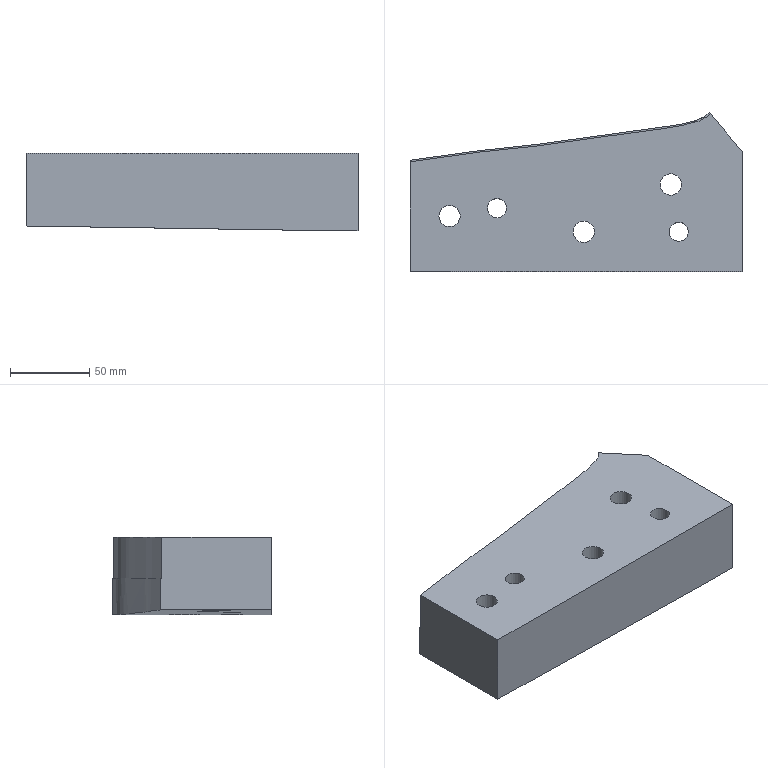Part | NX | features solid 2 | 1 solid | 25 faces | box 210 x 100.542 x 49 mm | volume 790054 mm3 | plane 13 | cylinder 10 | spline 2 | commonest cylinder face diameters 13.5 x3 19.5 x3 12 x2 13 x2
STEP:
#1=CARTESIAN_POINT('',(140.,-80.642,40.));
#2=VERTEX_POINT('',#1);
#3=CARTESIAN_POINT('',(329.994,-50.225,40.));
#4=VERTEX_POINT('',#3);
#5=CARTESIAN_POINT('',(140.,-80.642,40.));
#6=CARTESIAN_POINT('',(143.989,-80.088,40.));
#7=CARTESIAN_POINT('',(151.968,-78.986,40.));
#8=CARTESIAN_POINT('',(163.945,-77.392,40.));
#9=CARTESIAN_POINT('',(175.91,-75.711,40.));
#10=CARTESIAN_POINT('',(187.866,-73.962,40.));
#11=CARTESIAN_POINT('',(199.911,-72.906,40.));
#12=CARTESIAN_POINT('',(211.961,-71.887,40.));
#13=CARTESIAN_POINT('',(223.916,-70.128,40.));
#14=CARTESIAN_POINT('',(235.886,-68.491,40.));
#15=CARTESIAN_POINT('',(247.86,-66.876,40.));
#16=CARTESIAN_POINT('',(263.817,-64.665,40.));
#17=CARTESIAN_POINT('',(279.768,-62.407,40.));
#18=CARTESIAN_POINT('',(293.755,-60.651,40.));
#19=CARTESIAN_POINT('',(301.733,-59.549,40.));
#20=CARTESIAN_POINT('',(307.699,-58.616,40.));
#21=CARTESIAN_POINT('',(313.622,-57.464,40.));
#22=CARTESIAN_POINT('',(319.527,-56.12,40.));
#23=CARTESIAN_POINT('',(325.231,-54.225,40.));
#24=CARTESIAN_POINT('',(328.477,-51.599,40.));
#25=CARTESIAN_POINT('',(329.994,-50.225,40.));
#26=B_SPLINE_CURVE_WITH_KNOTS('',3,(#5,#6,#7,#8,#9,#10,#11,#12,#13,#14,#15,#16,#17,#18,#19,#20,#21,#22,#23,#24,#25),.UNSPECIFIED.,.F.,.F.,(4,1,1,1,1,1,1,1,1,1,1,1,1,1,1,1,1,1,4),(0.,0.01208,0.02416,0.03624,0.04833,0.06041,0.07249,0.08457,0.09665,0.1087,0.1208,0.145,0.1571,0.1631,0.1691,0.1752,0.1812,0.1873,0.1933),.UNSPECIFIED.);
#27=EDGE_CURVE('',#2,#4,#26,.T.);
#28=ORIENTED_EDGE('',*,*,#27,.F.);
#29=CARTESIAN_POINT('',(140.,-150.,40.));
#30=VERTEX_POINT('',#29);
#31=CARTESIAN_POINT('',(140.,35.09,40.));
#32=DIRECTION('',(0.,1.,0.));
#33=VECTOR('',#32,1000.);
#34=LINE('',#31,#33);
#35=EDGE_CURVE('',#30,#2,#34,.T.);
#36=ORIENTED_EDGE('',*,*,#35,.F.);
#37=CARTESIAN_POINT('',(350.,-150.,40.));
#38=VERTEX_POINT('',#37);
#39=CARTESIAN_POINT('',(-415.478,-150.,40.));
#40=DIRECTION('',(-1.,0.,0.));
#41=VECTOR('',#40,1000.);
#42=LINE('',#39,#41);
#43=EDGE_CURVE('',#38,#30,#42,.T.);
#44=ORIENTED_EDGE('',*,*,#43,.F.);
#45=CARTESIAN_POINT('',(350.,-74.067,40.));
#46=VERTEX_POINT('',#45);
#47=CARTESIAN_POINT('',(350.,35.09,40.));
#48=DIRECTION('',(0.,-1.,0.));
#49=VECTOR('',#48,1000.);
#50=LINE('',#47,#49);
#51=EDGE_CURVE('',#46,#38,#50,.T.);
#52=ORIENTED_EDGE('',*,*,#51,.F.);
#53=CARTESIAN_POINT('',(-20.026,366.913,40.));
#54=DIRECTION('',(-0.6428,0.766,0.));
#55=VECTOR('',#54,1000.);
#56=LINE('',#53,#55);
#57=EDGE_CURVE('',#46,#4,#56,.T.);
#58=ORIENTED_EDGE('',*,*,#57,.T.);
#59=EDGE_LOOP('',(#28,#36,#44,#52,#58));
#60=FACE_BOUND('',#59,.T.);
#61=CARTESIAN_POINT('',(316.,-125.,40.));
#62=VERTEX_POINT('',#61);
#63=CARTESIAN_POINT('',(310.,-125.,40.));
#64=DIRECTION('',(0.,0.,1.));
#65=DIRECTION('',(1.,0.,0.));
#66=AXIS2_PLACEMENT_3D('',#63,#64,#65);
#67=CIRCLE('',#66,6.);
#68=EDGE_CURVE('',#62,#62,#67,.T.);
#69=ORIENTED_EDGE('',*,*,#68,.F.);
#70=EDGE_LOOP('',(#69));
#71=FACE_BOUND('',#70,.T.);
#72=CARTESIAN_POINT('',(201.,-110.,40.));
#73=VERTEX_POINT('',#72);
#74=CARTESIAN_POINT('',(195.,-110.,40.));
#75=DIRECTION('',(0.,0.,1.));
#76=DIRECTION('',(1.,0.,0.));
#77=AXIS2_PLACEMENT_3D('',#74,#75,#76);
#78=CIRCLE('',#77,6.);
#79=EDGE_CURVE('',#73,#73,#78,.T.);
#80=ORIENTED_EDGE('',*,*,#79,.F.);
#81=EDGE_LOOP('',(#80));
#82=FACE_BOUND('',#81,.T.);
#83=CARTESIAN_POINT('',(256.75,-125.,40.));
#84=VERTEX_POINT('',#83);
#85=CARTESIAN_POINT('',(250.,-125.,40.));
#86=DIRECTION('',(0.,0.,1.));
#87=DIRECTION('',(1.,0.,0.));
#88=AXIS2_PLACEMENT_3D('',#85,#86,#87);
#89=CIRCLE('',#88,6.75);
#90=EDGE_CURVE('',#84,#84,#89,.T.);
#91=ORIENTED_EDGE('',*,*,#90,.F.);
#92=EDGE_LOOP('',(#91));
#93=FACE_BOUND('',#92,.T.);
#94=CARTESIAN_POINT('',(311.75,-95.,40.));
#95=VERTEX_POINT('',#94);
#96=CARTESIAN_POINT('',(305.,-95.,40.));
#97=DIRECTION('',(0.,0.,1.));
#98=DIRECTION('',(1.,0.,0.));
#99=AXIS2_PLACEMENT_3D('',#96,#97,#98);
#100=CIRCLE('',#99,6.75);
#101=EDGE_CURVE('',#95,#95,#100,.T.);
#102=ORIENTED_EDGE('',*,*,#101,.F.);
#103=EDGE_LOOP('',(#102));
#104=FACE_BOUND('',#103,.T.);
#105=CARTESIAN_POINT('',(171.75,-115.,40.));
#106=VERTEX_POINT('',#105);
#107=CARTESIAN_POINT('',(165.,-115.,40.));
#108=DIRECTION('',(0.,0.,1.));
#109=DIRECTION('',(1.,0.,0.));
#110=AXIS2_PLACEMENT_3D('',#107,#108,#109);
#111=CIRCLE('',#110,6.75);
#112=EDGE_CURVE('',#106,#106,#111,.T.);
#113=ORIENTED_EDGE('',*,*,#112,.F.);
#114=EDGE_LOOP('',(#113));
#115=FACE_BOUND('',#114,.T.);
#116=CARTESIAN_POINT('',(-415.478,35.09,40.));
#117=DIRECTION('',(0.,0.,1.));
#118=DIRECTION('',(1.,0.,0.));
#119=AXIS2_PLACEMENT_3D('',#116,#117,#118);
#120=PLANE('',#119);
#121=ADVANCED_FACE('',(#60,#71,#82,#93,#104,#115),#120,.T.);
#122=CARTESIAN_POINT('',(329.994,-50.225,14.));
#123=VERTEX_POINT('',#122);
#124=CARTESIAN_POINT('',(329.35,-49.458,14.));
#125=VERTEX_POINT('',#124);
#126=CARTESIAN_POINT('',(354.158,-79.022,14.));
#127=DIRECTION('',(-0.6428,0.766,0.));
#128=VECTOR('',#127,1000.);
#129=LINE('',#126,#128);
#130=EDGE_CURVE('',#123,#125,#129,.T.);
#131=ORIENTED_EDGE('',*,*,#130,.F.);
#132=CARTESIAN_POINT('',(329.994,-50.225,57.));
#133=DIRECTION('',(0.,0.,1.));
#134=VECTOR('',#133,1000.);
#135=LINE('',#132,#134);
#136=EDGE_CURVE('',#4,#123,#135,.F.);
#137=ORIENTED_EDGE('',*,*,#136,.F.);
#138=ORIENTED_EDGE('',*,*,#57,.F.);
#139=CARTESIAN_POINT('',(350.,-74.067,-9.));
#140=VERTEX_POINT('',#139);
#141=CARTESIAN_POINT('',(350.,-74.067,23.));
#142=DIRECTION('',(0.,0.,1.));
#143=VECTOR('',#142,1000.);
#144=LINE('',#141,#143);
#145=EDGE_CURVE('',#140,#46,#144,.T.);
#146=ORIENTED_EDGE('',*,*,#145,.F.);
#147=CARTESIAN_POINT('',(331.791,-52.366,-9.));
#148=VERTEX_POINT('',#147);
#149=CARTESIAN_POINT('',(83.881,243.081,-9.));
#150=DIRECTION('',(0.6428,-0.766,0.));
#151=VECTOR('',#150,1000.);
#152=LINE('',#149,#151);
#153=EDGE_CURVE('',#148,#140,#152,.T.);
#154=ORIENTED_EDGE('',*,*,#153,.F.);
#155=CARTESIAN_POINT('',(329.35,-49.458,-8.962));
#156=VERTEX_POINT('',#155);
#157=CARTESIAN_POINT('',(353.949,-78.773,-9.347));
#158=DIRECTION('',(-0.6428,0.766,0.01005));
#159=VECTOR('',#158,1000.);
#160=LINE('',#157,#159);
#161=EDGE_CURVE('',#148,#156,#160,.T.);
#162=ORIENTED_EDGE('',*,*,#161,.T.);
#163=CARTESIAN_POINT('',(329.35,-49.458,14.));
#164=DIRECTION('',(0.,0.,-1.));
#165=VECTOR('',#164,1000.);
#166=LINE('',#163,#165);
#167=EDGE_CURVE('',#125,#156,#166,.T.);
#168=ORIENTED_EDGE('',*,*,#167,.F.);
#169=EDGE_LOOP('',(#131,#137,#138,#146,#154,#162,#168));
#170=FACE_BOUND('',#169,.T.);
#171=CARTESIAN_POINT('',(354.158,-79.022,23.));
#172=DIRECTION('',(0.766,0.6428,0.));
#173=DIRECTION('',(-0.6428,0.766,0.));
#174=AXIS2_PLACEMENT_3D('',#171,#172,#173);
#175=PLANE('',#174);
#176=ADVANCED_FACE('',(#170),#175,.T.);
#177=CARTESIAN_POINT('',(140.,-150.,-6.));
#178=VERTEX_POINT('',#177);
#179=CARTESIAN_POINT('',(140.,-150.,2.));
#180=DIRECTION('',(0.,0.,-1.));
#181=VECTOR('',#180,1000.);
#182=LINE('',#179,#181);
#183=EDGE_CURVE('',#30,#178,#182,.T.);
#184=ORIENTED_EDGE('',*,*,#183,.T.);
#185=CARTESIAN_POINT('',(331.791,-150.,-9.));
#186=VERTEX_POINT('',#185);
#187=CARTESIAN_POINT('',(-470.232,-150.,3.545));
#188=DIRECTION('',(-0.9999,0.,0.01564));
#189=VECTOR('',#188,1000.);
#190=LINE('',#187,#189);
#191=EDGE_CURVE('',#186,#178,#190,.T.);
#192=ORIENTED_EDGE('',*,*,#191,.F.);
#193=CARTESIAN_POINT('',(350.,-150.,-9.));
#194=VERTEX_POINT('',#193);
#195=CARTESIAN_POINT('',(-470.381,-150.,-9.));
#196=DIRECTION('',(1.,0.,0.));
#197=VECTOR('',#196,1000.);
#198=LINE('',#195,#197);
#199=EDGE_CURVE('',#186,#194,#198,.T.);
#200=ORIENTED_EDGE('',*,*,#199,.T.);
#201=CARTESIAN_POINT('',(350.,-150.,2.));
#202=DIRECTION('',(0.,0.,1.));
#203=VECTOR('',#202,1000.);
#204=LINE('',#201,#203);
#205=EDGE_CURVE('',#194,#38,#204,.T.);
#206=ORIENTED_EDGE('',*,*,#205,.T.);
#207=ORIENTED_EDGE('',*,*,#43,.T.);
#208=EDGE_LOOP('',(#184,#192,#200,#206,#207));
#209=FACE_BOUND('',#208,.T.);
#210=CARTESIAN_POINT('',(0.,-150.,2.));
#211=DIRECTION('',(0.,1.,0.));
#212=DIRECTION('',(0.,0.,1.));
#213=AXIS2_PLACEMENT_3D('',#210,#211,#212);
#214=PLANE('',#213);
#215=ADVANCED_FACE('',(#209),#214,.F.);
#216=CARTESIAN_POINT('',(140.,-79.632,14.));
#217=VERTEX_POINT('',#216);
#218=CARTESIAN_POINT('',(-190.231,-121.49,14.));
#219=CARTESIAN_POINT('',(-188.654,-121.152,14.));
#220=CARTESIAN_POINT('',(-185.47,-120.627,14.));
#221=CARTESIAN_POINT('',(-180.656,-120.141,14.));
#222=CARTESIAN_POINT('',(-175.882,-119.326,14.));
#223=CARTESIAN_POINT('',(-169.679,-117.528,14.));
#224=CARTESIAN_POINT('',(-162.185,-114.539,14.));
#225=CARTESIAN_POINT('',(-153.086,-111.254,14.));
#226=CARTESIAN_POINT('',(-144.031,-107.845,14.));
#227=CARTESIAN_POINT('',(-136.465,-105.061,14.));
#228=CARTESIAN_POINT('',(-130.418,-102.814,14.));
#229=CARTESIAN_POINT('',(-125.812,-101.329,14.));
#230=CARTESIAN_POINT('',(-121.306,-99.566,14.));
#231=CARTESIAN_POINT('',(-116.876,-97.626,14.));
#232=CARTESIAN_POINT('',(-112.335,-95.923,14.));
#233=CARTESIAN_POINT('',(-107.564,-95.05,14.));
#234=CARTESIAN_POINT('',(-102.756,-94.525,14.));
#235=CARTESIAN_POINT('',(-96.349,-93.771,14.));
#236=CARTESIAN_POINT('',(-89.902,-93.468,14.));
#237=CARTESIAN_POINT('',(-83.452,-93.448,14.));
#238=CARTESIAN_POINT('',(-77.002,-93.469,14.));
#239=CARTESIAN_POINT('',(-68.939,-93.411,14.));
#240=CARTESIAN_POINT('',(-56.04,-93.3,14.));
#241=CARTESIAN_POINT('',(-33.465,-93.184,14.));
#242=CARTESIAN_POINT('',(-7.666,-93.074,14.));
#243=CARTESIAN_POINT('',(14.907,-92.653,14.));
#244=CARTESIAN_POINT('',(27.794,-92.068,14.));
#245=CARTESIAN_POINT('',(40.668,-91.245,14.));
#246=CARTESIAN_POINT('',(51.917,-90.291,14.));
#247=CARTESIAN_POINT('',(61.528,-89.174,14.));
#248=CARTESIAN_POINT('',(67.939,-88.466,14.));
#249=CARTESIAN_POINT('',(79.125,-86.95,14.));
#250=CARTESIAN_POINT('',(95.161,-85.253,14.));
#251=CARTESIAN_POINT('',(114.404,-83.21,14.));
#252=CARTESIAN_POINT('',(133.568,-80.524,14.));
#253=CARTESIAN_POINT('',(152.734,-77.861,14.));
#254=CARTESIAN_POINT('',(171.916,-75.326,14.));
#255=CARTESIAN_POINT('',(191.055,-72.413,14.));
#256=CARTESIAN_POINT('',(207.17,-71.468,14.));
#257=CARTESIAN_POINT('',(219.951,-69.697,14.));
#258=CARTESIAN_POINT('',(232.724,-67.899,14.));
#259=CARTESIAN_POINT('',(248.708,-65.766,14.));
#260=CARTESIAN_POINT('',(267.87,-63.074,14.));
#261=CARTESIAN_POINT('',(287.038,-60.44,14.));
#262=CARTESIAN_POINT('',(301.448,-58.682,14.));
#263=CARTESIAN_POINT('',(310.976,-56.987,14.));
#264=CARTESIAN_POINT('',(314.916,-56.135,14.));
#265=CARTESIAN_POINT('',(318.052,-55.382,14.));
#266=CARTESIAN_POINT('',(320.39,-54.76,14.));
#267=CARTESIAN_POINT('',(322.686,-53.981,14.));
#268=CARTESIAN_POINT('',(325.595,-52.578,14.));
#269=CARTESIAN_POINT('',(328.769,-50.098,14.));
#270=CARTESIAN_POINT('',(332.247,-46.69,14.));
#271=CARTESIAN_POINT('',(335.795,-43.406,14.));
#272=CARTESIAN_POINT('',(343.661,-37.758,14.));
#273=CARTESIAN_POINT('',(355.164,-28.914,14.));
#274=CARTESIAN_POINT('',(370.422,-17.018,14.));
#275=CARTESIAN_POINT('',(383.264,-7.249,14.));
#276=CARTESIAN_POINT('',(392.416,-0.6713,14.));
#277=CARTESIAN_POINT('',(396.953,2.733,14.));
#278=CARTESIAN_POINT('',(398.886,5.372,14.));
#279=CARTESIAN_POINT('',(399.725,7.654,14.));
#280=CARTESIAN_POINT('',(399.76,10.078,14.));
#281=CARTESIAN_POINT('',(399.483,13.317,14.));
#282=CARTESIAN_POINT('',(399.712,17.34,14.));
#283=CARTESIAN_POINT('',(399.612,22.179,14.));
#284=CARTESIAN_POINT('',(399.633,31.854,14.));
#285=CARTESIAN_POINT('',(399.593,46.366,14.));
#286=CARTESIAN_POINT('',(399.637,62.491,14.));
#287=CARTESIAN_POINT('',(399.588,73.779,14.));
#288=CARTESIAN_POINT('',(399.652,79.422,14.));
#289=CARTESIAN_POINT('',(399.59,82.647,14.));
#290=CARTESIAN_POINT('',(399.564,85.065,14.));
#291=CARTESIAN_POINT('',(399.725,87.486,14.));
#292=CARTESIAN_POINT('',(399.756,89.902,14.));
#293=CARTESIAN_POINT('',(399.247,92.301,14.));
#294=CARTESIAN_POINT('',(397.362,95.008,14.));
#295=CARTESIAN_POINT('',(393.635,96.774,14.));
#296=CARTESIAN_POINT('',(389.279,98.826,14.));
#297=CARTESIAN_POINT('',(384.732,100.498,14.));
#298=CARTESIAN_POINT('',(378.765,102.95,14.));
#299=CARTESIAN_POINT('',(362.589,110.229,14.));
#300=CARTESIAN_POINT('',(344.928,118.135,14.));
#301=CARTESIAN_POINT('',(327.281,126.072,14.));
#302=CARTESIAN_POINT('',(319.932,129.381,14.));
#303=CARTESIAN_POINT('',(314.075,132.102,14.));
#304=CARTESIAN_POINT('',(309.387,133.376,14.));
#305=CARTESIAN_POINT('',(304.547,133.785,14.));
#306=CARTESIAN_POINT('',(299.716,133.401,14.));
#307=CARTESIAN_POINT('',(294.929,132.704,14.));
#308=CARTESIAN_POINT('',(288.543,131.8,14.));
#309=CARTESIAN_POINT('',(277.364,130.241,14.));
#310=CARTESIAN_POINT('',(242.2,125.552,14.));
#311=CARTESIAN_POINT('',(184.637,118.048,14.));
#312=CARTESIAN_POINT('',(120.701,109.541,14.));
#313=CARTESIAN_POINT('',(69.531,102.902,14.));
#314=CARTESIAN_POINT('',(40.777,98.94,14.));
#315=CARTESIAN_POINT('',(21.566,96.615,14.));
#316=CARTESIAN_POINT('',(8.743,95.212,14.));
#317=CARTESIAN_POINT('',(-7.301,93.575,14.));
#318=CARTESIAN_POINT('',(-26.625,92.505,14.));
#319=CARTESIAN_POINT('',(-45.971,92.017,14.));
#320=CARTESIAN_POINT('',(-62.09,91.675,14.));
#321=CARTESIAN_POINT('',(-74.987,91.256,14.));
#322=CARTESIAN_POINT('',(-84.664,91.165,14.));
#323=CARTESIAN_POINT('',(-94.319,91.781,14.));
#324=CARTESIAN_POINT('',(-103.929,92.966,14.));
#325=CARTESIAN_POINT('',(-113.495,94.403,14.));
#326=CARTESIAN_POINT('',(-119.856,95.492,14.));
#327=CARTESIAN_POINT('',(-122.997,96.222,14.));
#328=B_SPLINE_CURVE_WITH_KNOTS('',3,(#218,#219,#220,#221,#222,#223,#224,#225,#226,#227,#228,#229,#230,#231,#232,#233,#234,#235,#236,#237,#238,#239,#240,#241,#242,#243,#244,#245,#246,#247,#248,#249,#250,#251,#252,#253,#254,#255,#256,#257,#258,#259,#260,#261,#262,#263,#264,#265,#266,#267,#268,#269,#270,#271,#272,#273,#274,#275,#276,#277,#278,#279,#280,#281,#282,#283,#284,#285,#286,#287,#288,#289,#290,#291,#292,#293,#294,#295,#296,#297,#298,#299,#300,#301,#302,#303,#304,#305,#306,#307,#308,#309,#310,#311,#312,#313,#314,#315,#316,#317,#318,#319,#320,#321,#322,#323,#324,#325,#326,#327),.UNSPECIFIED.,.F.,.F.,(4,1,1,1,1,1,1,1,1,1,1,1,1,1,1,1,1,1,1,1,1,1,1,1,1,1,1,1,1,1,1,1,1,1,1,1,1,1,1,1,1,1,1,1,1,1,1,1,1,1,1,1,1,1,1,1,1,1,1,1,1,1,1,1,1,1,1,1,1,1,1,1,1,1,1,1,1,1,1,1,1,1,1,1,1,1,1,1,1,1,1,1,1,1,1,1,1,1,1,1,1,1,1,1,1,1,1,4),(0.4704,0.4724,0.4745,0.4766,0.4786,0.4828,0.4869,0.491,0.4952,0.4972,0.4993,0.5014,0.5035,0.5055,0.5076,0.5097,0.5117,0.5159,0.5179,0.52,0.5241,0.5283,0.5366,0.5531,0.5614,0.5655,0.5697,0.5779,0.58,0.5821,0.5862,0.5945,0.6028,0.611,0.6193,0.6276,0.6359,0.6441,0.6483,0.6524,0.6607,0.669,0.6772,0.6855,0.6876,0.6897,0.6907,0.6917,0.6928,0.6938,0.6959,0.6979,0.7,0.7021,0.7103,0.7186,0.7269,0.731,0.7331,0.7341,0.7352,0.7362,0.7372,0.7393,0.7414,0.7435,0.7517,0.76,0.7641,0.7662,0.7672,0.7683,0.7693,0.7703,0.7714,0.7724,0.7745,0.7766,0.7786,0.7807,0.7848,0.8014,0.8055,0.8097,0.8117,0.8138,0.8159,0.8179,0.82,0.8221,0.8262,0.8345,0.8676,0.9007,0.9172,0.9338,0.9379,0.9421,0.9503,0.9586,0.9669,0.9752,0.9793,0.9834,0.9876,0.9917,0.9959,1.),.UNSPECIFIED.);
#329=EDGE_CURVE('',#125,#217,#328,.F.);
#330=ORIENTED_EDGE('',*,*,#329,.F.);
#331=ORIENTED_EDGE('',*,*,#167,.T.);
#332=CARTESIAN_POINT('',(140.,-79.632,-6.));
#333=VERTEX_POINT('',#332);
#334=CARTESIAN_POINT('',(140.,-79.632,-6.));
#335=CARTESIAN_POINT('',(143.987,-79.079,-6.062));
#336=CARTESIAN_POINT('',(151.962,-77.977,-6.187));
#337=CARTESIAN_POINT('',(163.931,-76.385,-6.374));
#338=CARTESIAN_POINT('',(175.889,-74.703,-6.561));
#339=CARTESIAN_POINT('',(191.822,-72.372,-6.811));
#340=CARTESIAN_POINT('',(207.937,-71.466,-7.063));
#341=CARTESIAN_POINT('',(223.862,-69.126,-7.312));
#342=CARTESIAN_POINT('',(235.822,-67.49,-7.499));
#343=CARTESIAN_POINT('',(247.785,-65.877,-7.686));
#344=CARTESIAN_POINT('',(263.728,-63.667,-7.935));
#345=CARTESIAN_POINT('',(279.664,-61.412,-8.185));
#346=CARTESIAN_POINT('',(293.642,-59.658,-8.403));
#347=CARTESIAN_POINT('',(301.613,-58.556,-8.528));
#348=CARTESIAN_POINT('',(307.579,-57.623,-8.621));
#349=CARTESIAN_POINT('',(313.493,-56.466,-8.714));
#350=CARTESIAN_POINT('',(319.444,-55.123,-8.807));
#351=CARTESIAN_POINT('',(325.005,-53.181,-8.894));
#352=CARTESIAN_POINT('',(327.933,-50.744,-8.94));
#353=CARTESIAN_POINT('',(329.35,-49.458,-8.962));
#354=B_SPLINE_CURVE_WITH_KNOTS('',3,(#334,#335,#336,#337,#338,#339,#340,#341,#342,#343,#344,#345,#346,#347,#348,#349,#350,#351,#352,#353),.UNSPECIFIED.,.F.,.F.,(4,1,1,1,1,1,1,1,1,1,1,1,1,1,1,1,1,4),(0.6815,0.6936,0.7058,0.7179,0.73,0.7542,0.7663,0.7785,0.7906,0.8027,0.8269,0.8391,0.8451,0.8512,0.8572,0.8633,0.8694,0.8754),.UNSPECIFIED.);
#355=EDGE_CURVE('',#156,#333,#354,.F.);
#356=ORIENTED_EDGE('',*,*,#355,.T.);
#357=CARTESIAN_POINT('',(140.,-79.632,27.));
#358=DIRECTION('',(0.,0.,-1.));
#359=VECTOR('',#358,1000.);
#360=LINE('',#357,#359);
#361=EDGE_CURVE('',#217,#333,#360,.T.);
#362=ORIENTED_EDGE('',*,*,#361,.F.);
#363=EDGE_LOOP('',(#330,#331,#356,#362));
#364=FACE_BOUND('',#363,.T.);
#365=CARTESIAN_POINT('',(140.,-79.632,14.));
#366=CARTESIAN_POINT('',(140.,-79.632,-9.1));
#367=CARTESIAN_POINT('',(143.976,-79.08,14.));
#368=CARTESIAN_POINT('',(143.976,-79.08,-9.1));
#369=CARTESIAN_POINT('',(151.93,-77.982,14.));
#370=CARTESIAN_POINT('',(151.93,-77.982,-9.1));
#371=CARTESIAN_POINT('',(163.867,-76.394,14.));
#372=CARTESIAN_POINT('',(163.867,-76.394,-9.1));
#373=CARTESIAN_POINT('',(175.795,-74.717,14.));
#374=CARTESIAN_POINT('',(175.795,-74.717,-9.1));
#375=CARTESIAN_POINT('',(187.715,-72.975,14.));
#376=CARTESIAN_POINT('',(187.715,-72.975,-9.1));
#377=CARTESIAN_POINT('',(199.711,-71.917,14.));
#378=CARTESIAN_POINT('',(199.711,-71.917,-9.1));
#379=CARTESIAN_POINT('',(211.715,-70.91,14.));
#380=CARTESIAN_POINT('',(211.715,-70.91,-9.1));
#381=CARTESIAN_POINT('',(223.635,-69.158,14.));
#382=CARTESIAN_POINT('',(223.635,-69.158,-9.1));
#383=CARTESIAN_POINT('',(235.566,-67.525,14.));
#384=CARTESIAN_POINT('',(235.566,-67.525,-9.1));
#385=CARTESIAN_POINT('',(247.502,-65.916,14.));
#386=CARTESIAN_POINT('',(247.502,-65.916,-9.1));
#387=CARTESIAN_POINT('',(263.408,-63.713,14.));
#388=CARTESIAN_POINT('',(263.408,-63.713,-9.1));
#389=CARTESIAN_POINT('',(279.306,-61.461,14.));
#390=CARTESIAN_POINT('',(279.306,-61.461,-9.1));
#391=CARTESIAN_POINT('',(293.249,-59.707,14.));
#392=CARTESIAN_POINT('',(293.249,-59.707,-9.1));
#393=CARTESIAN_POINT('',(301.203,-58.616,14.));
#394=CARTESIAN_POINT('',(301.203,-58.616,-9.1));
#395=CARTESIAN_POINT('',(307.153,-57.694,14.));
#396=CARTESIAN_POINT('',(307.153,-57.694,-9.1));
#397=CARTESIAN_POINT('',(313.072,-56.56,14.));
#398=CARTESIAN_POINT('',(313.072,-56.56,-9.1));
#399=CARTESIAN_POINT('',(318.933,-55.237,14.));
#400=CARTESIAN_POINT('',(318.933,-55.237,-9.1));
#401=CARTESIAN_POINT('',(324.733,-53.372,14.));
#402=CARTESIAN_POINT('',(324.733,-53.372,-9.1));
#403=CARTESIAN_POINT('',(327.86,-50.81,14.));
#404=CARTESIAN_POINT('',(327.86,-50.81,-9.1));
#405=CARTESIAN_POINT('',(329.35,-49.458,14.));
#406=CARTESIAN_POINT('',(329.35,-49.458,-9.1));
#407=B_SPLINE_SURFACE_WITH_KNOTS('',3,1,((#365,#366),(#367,#368),(#369,#370),(#371,#372),(#373,#374),(#375,#376),(#377,#378),(#379,#380),(#381,#382),(#383,#384),(#385,#386),(#387,#388),(#389,#390),(#391,#392),(#393,#394),(#395,#396),(#397,#398),(#399,#400),(#401,#402),(#403,#404),(#405,#406)),.SURF_OF_LINEAR_EXTRUSION.,.F.,.F.,.F.,(4,1,1,1,1,1,1,1,1,1,1,1,1,1,1,1,1,1,4),(2,2),(0.6138,0.619,0.6241,0.6293,0.6344,0.6396,0.6447,0.6499,0.655,0.6602,0.6653,0.6756,0.6808,0.6834,0.6859,0.6885,0.6911,0.6937,0.6962),(0.,1.),.UNSPECIFIED.);
#408=ADVANCED_FACE('',(#364),#407,.T.);
#409=ORIENTED_EDGE('',*,*,#205,.F.);
#410=CARTESIAN_POINT('',(350.,-222.,-9.));
#411=DIRECTION('',(0.,1.,0.));
#412=VECTOR('',#411,1000.);
#413=LINE('',#410,#412);
#414=EDGE_CURVE('',#194,#140,#413,.T.);
#415=ORIENTED_EDGE('',*,*,#414,.T.);
#416=ORIENTED_EDGE('',*,*,#145,.T.);
#417=ORIENTED_EDGE('',*,*,#51,.T.);
#418=EDGE_LOOP('',(#409,#415,#416,#417));
#419=FACE_BOUND('',#418,.T.);
#420=CARTESIAN_POINT('',(350.,-50.,2.));
#421=DIRECTION('',(-1.,0.,0.));
#422=DIRECTION('',(0.,0.,1.));
#423=AXIS2_PLACEMENT_3D('',#420,#421,#422);
#424=PLANE('',#423);
#425=ADVANCED_FACE('',(#419),#424,.F.);
#426=CARTESIAN_POINT('',(140.,-80.642,14.));
#427=VERTEX_POINT('',#426);
#428=CARTESIAN_POINT('',(140.,-80.642,57.));
#429=DIRECTION('',(0.,0.,1.));
#430=VECTOR('',#429,1000.);
#431=LINE('',#428,#430);
#432=EDGE_CURVE('',#2,#427,#431,.F.);
#433=ORIENTED_EDGE('',*,*,#432,.T.);
#434=CARTESIAN_POINT('',(140.,-115.282,14.));
#435=DIRECTION('',(0.,1.,0.));
#436=VECTOR('',#435,1000.);
#437=LINE('',#434,#436);
#438=EDGE_CURVE('',#427,#217,#437,.T.);
#439=ORIENTED_EDGE('',*,*,#438,.T.);
#440=ORIENTED_EDGE('',*,*,#361,.T.);
#441=CARTESIAN_POINT('',(140.,-222.,-6.));
#442=DIRECTION('',(0.,-1.,0.));
#443=VECTOR('',#442,1000.);
#444=LINE('',#441,#443);
#445=EDGE_CURVE('',#333,#178,#444,.T.);
#446=ORIENTED_EDGE('',*,*,#445,.T.);
#447=ORIENTED_EDGE('',*,*,#183,.F.);
#448=ORIENTED_EDGE('',*,*,#35,.T.);
#449=EDGE_LOOP('',(#433,#439,#440,#446,#447,#448));
#450=FACE_BOUND('',#449,.T.);
#451=CARTESIAN_POINT('',(140.,-115.282,21.5));
#452=DIRECTION('',(1.,0.,0.));
#453=DIRECTION('',(0.,0.,-1.));
#454=AXIS2_PLACEMENT_3D('',#451,#452,#453);
#455=PLANE('',#454);
#456=ADVANCED_FACE('',(#450),#455,.F.);
#457=ORIENTED_EDGE('',*,*,#112,.T.);
#458=EDGE_LOOP('',(#457));
#459=FACE_BOUND('',#458,.T.);
#460=CARTESIAN_POINT('',(171.75,-115.,9.));
#461=VERTEX_POINT('',#460);
#462=CARTESIAN_POINT('',(165.,-115.,9.));
#463=DIRECTION('',(0.,0.,1.));
#464=DIRECTION('',(1.,0.,0.));
#465=AXIS2_PLACEMENT_3D('',#462,#463,#464);
#466=CIRCLE('',#465,6.75);
#467=EDGE_CURVE('',#461,#461,#466,.T.);
#468=ORIENTED_EDGE('',*,*,#467,.F.);
#469=EDGE_LOOP('',(#468));
#470=FACE_BOUND('',#469,.T.);
#471=CARTESIAN_POINT('',(165.,-115.,94.));
#472=DIRECTION('',(0.,0.,1.));
#473=DIRECTION('',(1.,0.,0.));
#474=AXIS2_PLACEMENT_3D('',#471,#472,#473);
#475=CYLINDRICAL_SURFACE('',#474,6.75);
#476=ADVANCED_FACE('',(#459,#470),#475,.F.);
#477=ORIENTED_EDGE('',*,*,#467,.T.);
#478=EDGE_LOOP('',(#477));
#479=FACE_BOUND('',#478,.T.);
#480=CARTESIAN_POINT('',(174.75,-115.,9.));
#481=VERTEX_POINT('',#480);
#482=CARTESIAN_POINT('',(165.,-115.,9.));
#483=DIRECTION('',(0.,0.,1.));
#484=DIRECTION('',(1.,0.,0.));
#485=AXIS2_PLACEMENT_3D('',#482,#483,#484);
#486=CIRCLE('',#485,9.75);
#487=EDGE_CURVE('',#481,#481,#486,.T.);
#488=ORIENTED_EDGE('',*,*,#487,.F.);
#489=EDGE_LOOP('',(#488));
#490=FACE_BOUND('',#489,.T.);
#491=CARTESIAN_POINT('',(165.,-115.,9.));
#492=DIRECTION('',(0.,0.,1.));
#493=DIRECTION('',(1.,0.,0.));
#494=AXIS2_PLACEMENT_3D('',#491,#492,#493);
#495=PLANE('',#494);
#496=ADVANCED_FACE('',(#479,#490),#495,.F.);
#497=ORIENTED_EDGE('',*,*,#487,.T.);
#498=EDGE_LOOP('',(#497));
#499=FACE_BOUND('',#498,.T.);
#500=CARTESIAN_POINT('',(174.75,-115.,-6.544));
#501=VERTEX_POINT('',#500);
#502=CARTESIAN_POINT('',(165.,-115.,-6.391));
#503=DIRECTION('',(-0.01564,0.,-0.9999));
#504=DIRECTION('',(0.9999,0.,-0.01564));
#505=AXIS2_PLACEMENT_3D('',#502,#503,#504);
#506=ELLIPSE('',#505,9.751,9.75);
#507=EDGE_CURVE('',#501,#501,#506,.T.);
#508=ORIENTED_EDGE('',*,*,#507,.T.);
#509=EDGE_LOOP('',(#508));
#510=FACE_BOUND('',#509,.T.);
#511=CARTESIAN_POINT('',(165.,-115.,-6.));
#512=DIRECTION('',(0.,0.,1.));
#513=DIRECTION('',(1.,0.,0.));
#514=AXIS2_PLACEMENT_3D('',#511,#512,#513);
#515=CYLINDRICAL_SURFACE('',#514,9.75);
#516=ADVANCED_FACE('',(#499,#510),#515,.F.);
#517=ORIENTED_EDGE('',*,*,#101,.T.);
#518=EDGE_LOOP('',(#517));
#519=FACE_BOUND('',#518,.T.);
#520=CARTESIAN_POINT('',(311.75,-95.,9.));
#521=VERTEX_POINT('',#520);
#522=CARTESIAN_POINT('',(305.,-95.,9.));
#523=DIRECTION('',(0.,0.,1.));
#524=DIRECTION('',(1.,0.,0.));
#525=AXIS2_PLACEMENT_3D('',#522,#523,#524);
#526=CIRCLE('',#525,6.75);
#527=EDGE_CURVE('',#521,#521,#526,.T.);
#528=ORIENTED_EDGE('',*,*,#527,.F.);
#529=EDGE_LOOP('',(#528));
#530=FACE_BOUND('',#529,.T.);
#531=CARTESIAN_POINT('',(305.,-95.,94.));
#532=DIRECTION('',(0.,0.,1.));
#533=DIRECTION('',(1.,0.,0.));
#534=AXIS2_PLACEMENT_3D('',#531,#532,#533);
#535=CYLINDRICAL_SURFACE('',#534,6.75);
#536=ADVANCED_FACE('',(#519,#530),#535,.F.);
#537=ORIENTED_EDGE('',*,*,#527,.T.);
#538=EDGE_LOOP('',(#537));
#539=FACE_BOUND('',#538,.T.);
#540=CARTESIAN_POINT('',(314.75,-95.,9.));
#541=VERTEX_POINT('',#540);
#542=CARTESIAN_POINT('',(305.,-95.,9.));
#543=DIRECTION('',(0.,0.,1.));
#544=DIRECTION('',(1.,0.,0.));
#545=AXIS2_PLACEMENT_3D('',#542,#543,#544);
#546=CIRCLE('',#545,9.75);
#547=EDGE_CURVE('',#541,#541,#546,.T.);
#548=ORIENTED_EDGE('',*,*,#547,.F.);
#549=EDGE_LOOP('',(#548));
#550=FACE_BOUND('',#549,.T.);
#551=CARTESIAN_POINT('',(305.,-95.,9.));
#552=DIRECTION('',(0.,0.,1.));
#553=DIRECTION('',(1.,0.,0.));
#554=AXIS2_PLACEMENT_3D('',#551,#552,#553);
#555=PLANE('',#554);
#556=ADVANCED_FACE('',(#539,#550),#555,.F.);
#557=ORIENTED_EDGE('',*,*,#547,.T.);
#558=EDGE_LOOP('',(#557));
#559=FACE_BOUND('',#558,.T.);
#560=CARTESIAN_POINT('',(314.75,-95.,-8.733));
#561=VERTEX_POINT('',#560);
#562=CARTESIAN_POINT('',(305.,-95.,-8.581));
#563=DIRECTION('',(-0.01564,0.,-0.9999));
#564=DIRECTION('',(0.9999,0.,-0.01564));
#565=AXIS2_PLACEMENT_3D('',#562,#563,#564);
#566=ELLIPSE('',#565,9.751,9.75);
#567=EDGE_CURVE('',#561,#561,#566,.T.);
#568=ORIENTED_EDGE('',*,*,#567,.T.);
#569=EDGE_LOOP('',(#568));
#570=FACE_BOUND('',#569,.T.);
#571=CARTESIAN_POINT('',(305.,-95.,-6.));
#572=DIRECTION('',(0.,0.,1.));
#573=DIRECTION('',(1.,0.,0.));
#574=AXIS2_PLACEMENT_3D('',#571,#572,#573);
#575=CYLINDRICAL_SURFACE('',#574,9.75);
#576=ADVANCED_FACE('',(#559,#570),#575,.F.);
#577=ORIENTED_EDGE('',*,*,#90,.T.);
#578=EDGE_LOOP('',(#577));
#579=FACE_BOUND('',#578,.T.);
#580=CARTESIAN_POINT('',(256.75,-125.,9.));
#581=VERTEX_POINT('',#580);
#582=CARTESIAN_POINT('',(250.,-125.,9.));
#583=DIRECTION('',(0.,0.,1.));
#584=DIRECTION('',(1.,0.,0.));
#585=AXIS2_PLACEMENT_3D('',#582,#583,#584);
#586=CIRCLE('',#585,6.75);
#587=EDGE_CURVE('',#581,#581,#586,.T.);
#588=ORIENTED_EDGE('',*,*,#587,.F.);
#589=EDGE_LOOP('',(#588));
#590=FACE_BOUND('',#589,.T.);
#591=CARTESIAN_POINT('',(250.,-125.,94.));
#592=DIRECTION('',(0.,0.,1.));
#593=DIRECTION('',(1.,0.,0.));
#594=AXIS2_PLACEMENT_3D('',#591,#592,#593);
#595=CYLINDRICAL_SURFACE('',#594,6.75);
#596=ADVANCED_FACE('',(#579,#590),#595,.F.);
#597=ORIENTED_EDGE('',*,*,#587,.T.);
#598=EDGE_LOOP('',(#597));
#599=FACE_BOUND('',#598,.T.);
#600=CARTESIAN_POINT('',(259.75,-125.,9.));
#601=VERTEX_POINT('',#600);
#602=CARTESIAN_POINT('',(250.,-125.,9.));
#603=DIRECTION('',(0.,0.,1.));
#604=DIRECTION('',(1.,0.,0.));
#605=AXIS2_PLACEMENT_3D('',#602,#603,#604);
#606=CIRCLE('',#605,9.75);
#607=EDGE_CURVE('',#601,#601,#606,.T.);
#608=ORIENTED_EDGE('',*,*,#607,.F.);
#609=EDGE_LOOP('',(#608));
#610=FACE_BOUND('',#609,.T.);
#611=CARTESIAN_POINT('',(250.,-125.,9.));
#612=DIRECTION('',(0.,0.,1.));
#613=DIRECTION('',(1.,0.,0.));
#614=AXIS2_PLACEMENT_3D('',#611,#612,#613);
#615=PLANE('',#614);
#616=ADVANCED_FACE('',(#599,#610),#615,.F.);
#617=ORIENTED_EDGE('',*,*,#607,.T.);
#618=EDGE_LOOP('',(#617));
#619=FACE_BOUND('',#618,.T.);
#620=CARTESIAN_POINT('',(259.75,-125.,-7.873));
#621=VERTEX_POINT('',#620);
#622=CARTESIAN_POINT('',(250.,-125.,-7.721));
#623=DIRECTION('',(-0.01564,0.,-0.9999));
#624=DIRECTION('',(0.9999,0.,-0.01564));
#625=AXIS2_PLACEMENT_3D('',#622,#623,#624);
#626=ELLIPSE('',#625,9.751,9.75);
#627=EDGE_CURVE('',#621,#621,#626,.T.);
#628=ORIENTED_EDGE('',*,*,#627,.T.);
#629=EDGE_LOOP('',(#628));
#630=FACE_BOUND('',#629,.T.);
#631=CARTESIAN_POINT('',(250.,-125.,-6.));
#632=DIRECTION('',(0.,0.,1.));
#633=DIRECTION('',(1.,0.,0.));
#634=AXIS2_PLACEMENT_3D('',#631,#632,#633);
#635=CYLINDRICAL_SURFACE('',#634,9.75);
#636=ADVANCED_FACE('',(#619,#630),#635,.F.);
#637=ORIENTED_EDGE('',*,*,#79,.T.);
#638=EDGE_LOOP('',(#637));
#639=FACE_BOUND('',#638,.T.);
#640=CARTESIAN_POINT('',(201.,-110.,14.));
#641=VERTEX_POINT('',#640);
#642=CARTESIAN_POINT('',(195.,-110.,14.));
#643=DIRECTION('',(0.,0.,1.));
#644=DIRECTION('',(1.,0.,0.));
#645=AXIS2_PLACEMENT_3D('',#642,#643,#644);
#646=CIRCLE('',#645,6.);
#647=EDGE_CURVE('',#641,#641,#646,.T.);
#648=ORIENTED_EDGE('',*,*,#647,.F.);
#649=EDGE_LOOP('',(#648));
#650=FACE_BOUND('',#649,.T.);
#651=CARTESIAN_POINT('',(195.,-110.,94.));
#652=DIRECTION('',(0.,0.,1.));
#653=DIRECTION('',(1.,0.,0.));
#654=AXIS2_PLACEMENT_3D('',#651,#652,#653);
#655=CYLINDRICAL_SURFACE('',#654,6.);
#656=ADVANCED_FACE('',(#639,#650),#655,.F.);
#657=ORIENTED_EDGE('',*,*,#647,.T.);
#658=EDGE_LOOP('',(#657));
#659=FACE_BOUND('',#658,.T.);
#660=CARTESIAN_POINT('',(201.5,-110.,14.));
#661=VERTEX_POINT('',#660);
#662=CARTESIAN_POINT('',(195.,-110.,14.));
#663=DIRECTION('',(0.,0.,1.));
#664=DIRECTION('',(1.,0.,0.));
#665=AXIS2_PLACEMENT_3D('',#662,#663,#664);
#666=CIRCLE('',#665,6.5);
#667=EDGE_CURVE('',#661,#661,#666,.T.);
#668=ORIENTED_EDGE('',*,*,#667,.F.);
#669=EDGE_LOOP('',(#668));
#670=FACE_BOUND('',#669,.T.);
#671=CARTESIAN_POINT('',(195.,-115.,14.));
#672=DIRECTION('',(0.,0.,1.));
#673=DIRECTION('',(1.,0.,0.));
#674=AXIS2_PLACEMENT_3D('',#671,#672,#673);
#675=PLANE('',#674);
#676=ADVANCED_FACE('',(#659,#670),#675,.F.);
#677=ORIENTED_EDGE('',*,*,#667,.T.);
#678=EDGE_LOOP('',(#677));
#679=FACE_BOUND('',#678,.T.);
#680=CARTESIAN_POINT('',(201.5,-110.,-6.962));
#681=VERTEX_POINT('',#680);
#682=CARTESIAN_POINT('',(195.,-110.,-6.86));
#683=DIRECTION('',(-0.01564,0.,-0.9999));
#684=DIRECTION('',(0.9999,0.,-0.01564));
#685=AXIS2_PLACEMENT_3D('',#682,#683,#684);
#686=ELLIPSE('',#685,6.501,6.5);
#687=EDGE_CURVE('',#681,#681,#686,.T.);
#688=ORIENTED_EDGE('',*,*,#687,.T.);
#689=EDGE_LOOP('',(#688));
#690=FACE_BOUND('',#689,.T.);
#691=CARTESIAN_POINT('',(195.,-110.,-6.));
#692=DIRECTION('',(0.,0.,1.));
#693=DIRECTION('',(1.,0.,0.));
#694=AXIS2_PLACEMENT_3D('',#691,#692,#693);
#695=CYLINDRICAL_SURFACE('',#694,6.5);
#696=ADVANCED_FACE('',(#679,#690),#695,.F.);
#697=ORIENTED_EDGE('',*,*,#68,.T.);
#698=EDGE_LOOP('',(#697));
#699=FACE_BOUND('',#698,.T.);
#700=CARTESIAN_POINT('',(316.,-125.,14.));
#701=VERTEX_POINT('',#700);
#702=CARTESIAN_POINT('',(310.,-125.,14.));
#703=DIRECTION('',(0.,0.,1.));
#704=DIRECTION('',(1.,0.,0.));
#705=AXIS2_PLACEMENT_3D('',#702,#703,#704);
#706=CIRCLE('',#705,6.);
#707=EDGE_CURVE('',#701,#701,#706,.T.);
#708=ORIENTED_EDGE('',*,*,#707,.F.);
#709=EDGE_LOOP('',(#708));
#710=FACE_BOUND('',#709,.T.);
#711=CARTESIAN_POINT('',(310.,-125.,94.));
#712=DIRECTION('',(0.,0.,1.));
#713=DIRECTION('',(1.,0.,0.));
#714=AXIS2_PLACEMENT_3D('',#711,#712,#713);
#715=CYLINDRICAL_SURFACE('',#714,6.);
#716=ADVANCED_FACE('',(#699,#710),#715,.F.);
#717=ORIENTED_EDGE('',*,*,#707,.T.);
#718=EDGE_LOOP('',(#717));
#719=FACE_BOUND('',#718,.T.);
#720=CARTESIAN_POINT('',(316.5,-125.,14.));
#721=VERTEX_POINT('',#720);
#722=CARTESIAN_POINT('',(310.,-125.,14.));
#723=DIRECTION('',(0.,0.,1.));
#724=DIRECTION('',(1.,0.,0.));
#725=AXIS2_PLACEMENT_3D('',#722,#723,#724);
#726=CIRCLE('',#725,6.5);
#727=EDGE_CURVE('',#721,#721,#726,.T.);
#728=ORIENTED_EDGE('',*,*,#727,.F.);
#729=EDGE_LOOP('',(#728));
#730=FACE_BOUND('',#729,.T.);
#731=CARTESIAN_POINT('',(310.,-125.,14.));
#732=DIRECTION('',(0.,0.,1.));
#733=DIRECTION('',(1.,0.,0.));
#734=AXIS2_PLACEMENT_3D('',#731,#732,#733);
#735=PLANE('',#734);
#736=ADVANCED_FACE('',(#719,#730),#735,.F.);
#737=ORIENTED_EDGE('',*,*,#727,.T.);
#738=EDGE_LOOP('',(#737));
#739=FACE_BOUND('',#738,.T.);
#740=CARTESIAN_POINT('',(316.5,-125.,-8.761));
#741=VERTEX_POINT('',#740);
#742=CARTESIAN_POINT('',(310.,-125.,-8.659));
#743=DIRECTION('',(-0.01564,0.,-0.9999));
#744=DIRECTION('',(0.9999,0.,-0.01564));
#745=AXIS2_PLACEMENT_3D('',#742,#743,#744);
#746=ELLIPSE('',#745,6.501,6.5);
#747=EDGE_CURVE('',#741,#741,#746,.T.);
#748=ORIENTED_EDGE('',*,*,#747,.T.);
#749=EDGE_LOOP('',(#748));
#750=FACE_BOUND('',#749,.T.);
#751=CARTESIAN_POINT('',(310.,-125.,-6.));
#752=DIRECTION('',(0.,0.,1.));
#753=DIRECTION('',(1.,0.,0.));
#754=AXIS2_PLACEMENT_3D('',#751,#752,#753);
#755=CYLINDRICAL_SURFACE('',#754,6.5);
#756=ADVANCED_FACE('',(#739,#750),#755,.F.);
#757=ORIENTED_EDGE('',*,*,#199,.F.);
#758=CARTESIAN_POINT('',(331.791,-222.,-9.));
#759=DIRECTION('',(0.,1.,0.));
#760=VECTOR('',#759,1000.);
#761=LINE('',#758,#760);
#762=EDGE_CURVE('',#186,#148,#761,.T.);
#763=ORIENTED_EDGE('',*,*,#762,.T.);
#764=ORIENTED_EDGE('',*,*,#153,.T.);
#765=ORIENTED_EDGE('',*,*,#414,.F.);
#766=EDGE_LOOP('',(#757,#763,#764,#765));
#767=FACE_BOUND('',#766,.T.);
#768=CARTESIAN_POINT('',(-470.381,-222.,-9.));
#769=DIRECTION('',(0.,0.,-1.));
#770=DIRECTION('',(-1.,0.,0.));
#771=AXIS2_PLACEMENT_3D('',#768,#769,#770);
#772=PLANE('',#771);
#773=ADVANCED_FACE('',(#767),#772,.T.);
#774=ORIENTED_EDGE('',*,*,#507,.F.);
#775=EDGE_LOOP('',(#774));
#776=FACE_BOUND('',#775,.T.);
#777=ORIENTED_EDGE('',*,*,#567,.F.);
#778=EDGE_LOOP('',(#777));
#779=FACE_BOUND('',#778,.T.);
#780=ORIENTED_EDGE('',*,*,#627,.F.);
#781=EDGE_LOOP('',(#780));
#782=FACE_BOUND('',#781,.T.);
#783=ORIENTED_EDGE('',*,*,#687,.F.);
#784=EDGE_LOOP('',(#783));
#785=FACE_BOUND('',#784,.T.);
#786=ORIENTED_EDGE('',*,*,#747,.F.);
#787=EDGE_LOOP('',(#786));
#788=FACE_BOUND('',#787,.T.);
#789=ORIENTED_EDGE('',*,*,#762,.F.);
#790=ORIENTED_EDGE('',*,*,#191,.T.);
#791=ORIENTED_EDGE('',*,*,#445,.F.);
#792=ORIENTED_EDGE('',*,*,#355,.F.);
#793=ORIENTED_EDGE('',*,*,#161,.F.);
#794=EDGE_LOOP('',(#789,#790,#791,#792,#793));
#795=FACE_BOUND('',#794,.T.);
#796=CARTESIAN_POINT('',(140.,-150.,-6.));
#797=DIRECTION('',(-0.01564,0.,-0.9999));
#798=DIRECTION('',(-0.9999,0.,0.01564));
#799=AXIS2_PLACEMENT_3D('',#796,#797,#798);
#800=PLANE('',#799);
#801=ADVANCED_FACE('',(#776,#779,#782,#785,#788,#795),#800,.T.);
#802=ORIENTED_EDGE('',*,*,#130,.T.);
#803=ORIENTED_EDGE('',*,*,#329,.T.);
#804=ORIENTED_EDGE('',*,*,#438,.F.);
#805=CARTESIAN_POINT('',(140.,-80.642,14.));
#806=CARTESIAN_POINT('',(143.978,-80.09,14.));
#807=CARTESIAN_POINT('',(151.933,-78.99,14.));
#808=CARTESIAN_POINT('',(163.874,-77.402,14.));
#809=CARTESIAN_POINT('',(175.826,-75.723,14.));
#810=CARTESIAN_POINT('',(187.729,-73.981,14.));
#811=CARTESIAN_POINT('',(199.666,-72.922,14.));
#812=CARTESIAN_POINT('',(211.739,-71.915,14.));
#813=CARTESIAN_POINT('',(223.685,-70.161,14.));
#814=CARTESIAN_POINT('',(235.611,-68.528,14.));
#815=CARTESIAN_POINT('',(247.555,-66.918,14.));
#816=CARTESIAN_POINT('',(263.475,-64.713,14.));
#817=CARTESIAN_POINT('',(279.376,-62.46,14.));
#818=CARTESIAN_POINT('',(293.315,-60.706,14.));
#819=CARTESIAN_POINT('',(301.294,-59.614,14.));
#820=CARTESIAN_POINT('',(307.267,-58.688,14.));
#821=CARTESIAN_POINT('',(313.239,-57.552,14.));
#822=CARTESIAN_POINT('',(318.142,-56.428,14.));
#823=CARTESIAN_POINT('',(322.105,-55.292,14.));
#824=CARTESIAN_POINT('',(326.024,-53.596,14.));
#825=CARTESIAN_POINT('',(328.475,-51.601,14.));
#826=CARTESIAN_POINT('',(329.994,-50.225,14.));
#827=B_SPLINE_CURVE_WITH_KNOTS('',3,(#805,#806,#807,#808,#809,#810,#811,#812,#813,#814,#815,#816,#817,#818,#819,#820,#821,#822,#823,#824,#825,#826),.UNSPECIFIED.,.F.,.F.,(4,1,1,1,1,1,1,1,1,1,1,1,1,1,1,1,1,1,1,4),(0.6138,0.6189,0.6241,0.6292,0.6344,0.6395,0.6447,0.6498,0.655,0.6601,0.6653,0.6756,0.6808,0.6833,0.6859,0.6885,0.6911,0.6923,0.6936,0.6962),.UNSPECIFIED.);
#828=EDGE_CURVE('',#427,#123,#827,.T.);
#829=ORIENTED_EDGE('',*,*,#828,.T.);
#830=EDGE_LOOP('',(#802,#803,#804,#829));
#831=FACE_BOUND('',#830,.T.);
#832=CARTESIAN_POINT('',(-190.231,-121.49,14.));
#833=DIRECTION('',(0.,0.,-1.));
#834=DIRECTION('',(-1.,0.,0.));
#835=AXIS2_PLACEMENT_3D('',#832,#833,#834);
#836=PLANE('',#835);
#837=ADVANCED_FACE('',(#831),#836,.F.);
#838=ORIENTED_EDGE('',*,*,#136,.T.);
#839=ORIENTED_EDGE('',*,*,#828,.F.);
#840=ORIENTED_EDGE('',*,*,#432,.F.);
#841=ORIENTED_EDGE('',*,*,#27,.T.);
#842=EDGE_LOOP('',(#838,#839,#840,#841));
#843=FACE_BOUND('',#842,.T.);
#844=CARTESIAN_POINT('',(140.,-80.642,14.));
#845=CARTESIAN_POINT('',(140.,-80.642,40.));
#846=CARTESIAN_POINT('',(143.978,-80.09,14.));
#847=CARTESIAN_POINT('',(143.978,-80.09,40.));
#848=CARTESIAN_POINT('',(151.933,-78.99,14.));
#849=CARTESIAN_POINT('',(151.933,-78.99,40.));
#850=CARTESIAN_POINT('',(163.874,-77.402,14.));
#851=CARTESIAN_POINT('',(163.874,-77.402,40.));
#852=CARTESIAN_POINT('',(175.826,-75.723,14.));
#853=CARTESIAN_POINT('',(175.826,-75.723,40.));
#854=CARTESIAN_POINT('',(187.729,-73.981,14.));
#855=CARTESIAN_POINT('',(187.729,-73.981,40.));
#856=CARTESIAN_POINT('',(199.666,-72.922,14.));
#857=CARTESIAN_POINT('',(199.666,-72.922,40.));
#858=CARTESIAN_POINT('',(211.739,-71.915,14.));
#859=CARTESIAN_POINT('',(211.739,-71.915,40.));
#860=CARTESIAN_POINT('',(223.685,-70.161,14.));
#861=CARTESIAN_POINT('',(223.685,-70.161,40.));
#862=CARTESIAN_POINT('',(235.611,-68.528,14.));
#863=CARTESIAN_POINT('',(235.611,-68.528,40.));
#864=CARTESIAN_POINT('',(247.555,-66.918,14.));
#865=CARTESIAN_POINT('',(247.555,-66.918,40.));
#866=CARTESIAN_POINT('',(263.475,-64.713,14.));
#867=CARTESIAN_POINT('',(263.475,-64.713,40.));
#868=CARTESIAN_POINT('',(279.376,-62.46,14.));
#869=CARTESIAN_POINT('',(279.376,-62.46,40.));
#870=CARTESIAN_POINT('',(293.315,-60.706,14.));
#871=CARTESIAN_POINT('',(293.315,-60.706,40.));
#872=CARTESIAN_POINT('',(301.294,-59.614,14.));
#873=CARTESIAN_POINT('',(301.294,-59.614,40.));
#874=CARTESIAN_POINT('',(307.267,-58.688,14.));
#875=CARTESIAN_POINT('',(307.267,-58.688,40.));
#876=CARTESIAN_POINT('',(313.239,-57.552,14.));
#877=CARTESIAN_POINT('',(313.239,-57.552,40.));
#878=CARTESIAN_POINT('',(318.142,-56.428,14.));
#879=CARTESIAN_POINT('',(318.142,-56.428,40.));
#880=CARTESIAN_POINT('',(322.105,-55.292,14.));
#881=CARTESIAN_POINT('',(322.105,-55.292,40.));
#882=CARTESIAN_POINT('',(326.024,-53.596,14.));
#883=CARTESIAN_POINT('',(326.024,-53.596,40.));
#884=CARTESIAN_POINT('',(328.475,-51.601,14.));
#885=CARTESIAN_POINT('',(328.475,-51.601,40.));
#886=CARTESIAN_POINT('',(329.994,-50.225,14.));
#887=CARTESIAN_POINT('',(329.994,-50.225,40.));
#888=B_SPLINE_SURFACE_WITH_KNOTS('',3,1,((#844,#845),(#846,#847),(#848,#849),(#850,#851),(#852,#853),(#854,#855),(#856,#857),(#858,#859),(#860,#861),(#862,#863),(#864,#865),(#866,#867),(#868,#869),(#870,#871),(#872,#873),(#874,#875),(#876,#877),(#878,#879),(#880,#881),(#882,#883),(#884,#885),(#886,#887)),.SURF_OF_LINEAR_EXTRUSION.,.F.,.F.,.F.,(4,1,1,1,1,1,1,1,1,1,1,1,1,1,1,1,1,1,1,4),(2,2),(0.6138,0.6189,0.6241,0.6292,0.6344,0.6395,0.6447,0.6498,0.655,0.6601,0.6653,0.6756,0.6808,0.6833,0.6859,0.6885,0.6911,0.6923,0.6936,0.6962),(0.,1.),.UNSPECIFIED.);
#889=ADVANCED_FACE('',(#843),#888,.F.);
#890=CLOSED_SHELL('',(#121,#176,#215,#408,#425,#456,#476,#496,#516,#536,#556,#576,#596,#616,#636,#656,#676,#696,#716,#736,#756,#773,#801,#837,#889));
#891=MANIFOLD_SOLID_BREP('',#890);
#892=(LENGTH_UNIT()NAMED_UNIT(*)SI_UNIT(.MILLI.,.METRE.));
#893=UNCERTAINTY_MEASURE_WITH_UNIT(LENGTH_MEASURE(0.0508),#892,'','');
#894=(NAMED_UNIT(*)PLANE_ANGLE_UNIT()SI_UNIT($,.RADIAN.));
#895=(NAMED_UNIT(*)SI_UNIT($,.STERADIAN.)SOLID_ANGLE_UNIT());
#896=(GEOMETRIC_REPRESENTATION_CONTEXT(3)GLOBAL_UNCERTAINTY_ASSIGNED_CONTEXT((#893))GLOBAL_UNIT_ASSIGNED_CONTEXT((#892,#894,#895))REPRESENTATION_CONTEXT('',''));
#897=ADVANCED_BREP_SHAPE_REPRESENTATION('',(#891),#896);